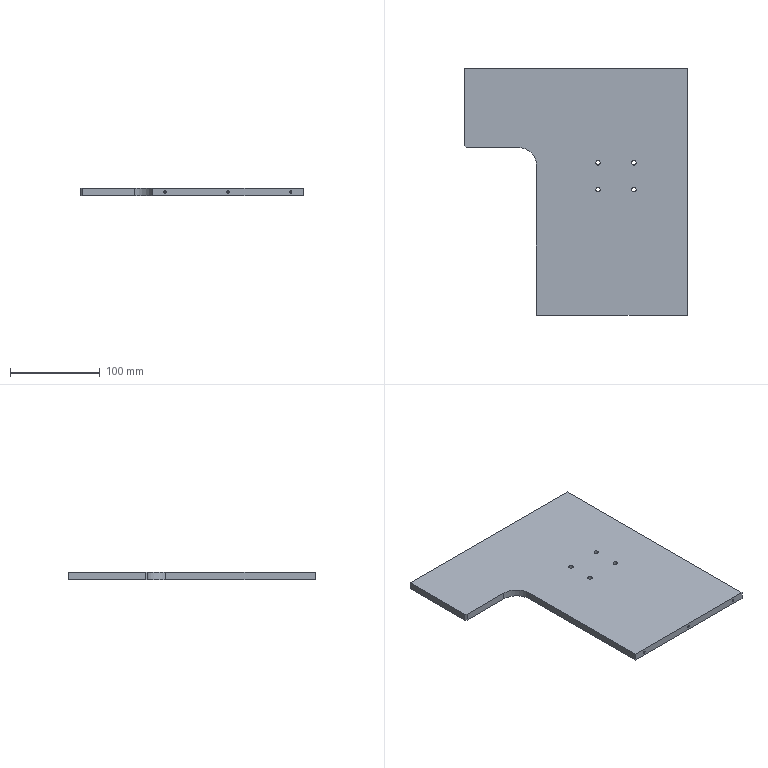Part | STEP file | CA-10-009Lift Stop Plate5_Default | 1 solid | 54 faces | box 248 x 275 x 8 mm | volume 425355 mm3 | cylinder 27 | cone 18 | plane 9 | commonest cylinder face diameters 2.5 x18 5 x8 40 x1